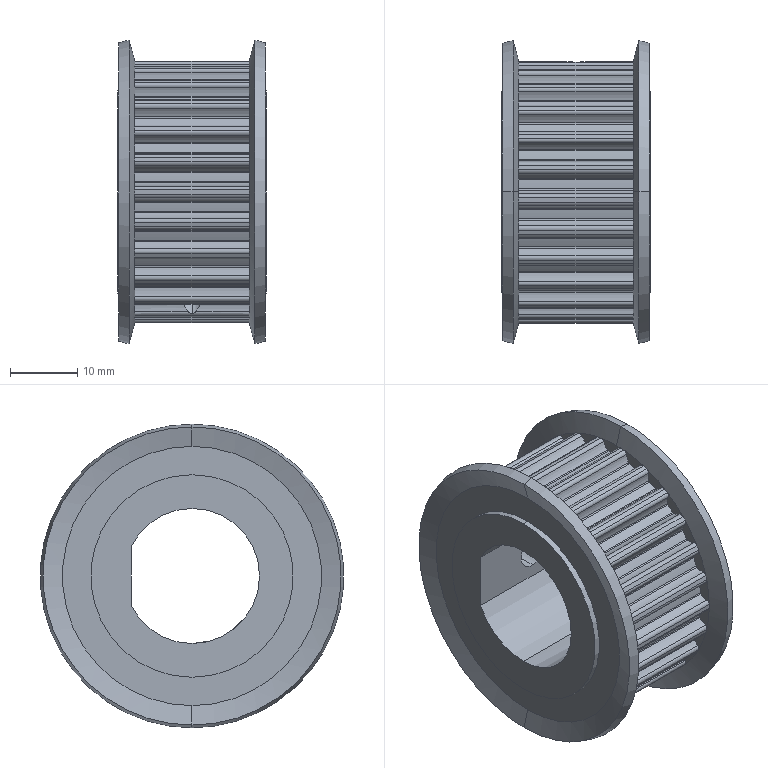Part | SolidWorks | features BaseBody 1 | 1 solid | 290 faces | box 22 x 45 x 45 mm | volume 17406 mm3 | cylinder 223 | plane 55 | cone 12 | commonest cylinder face diameters 0.5 x54 6.55 x54 1.1 x52 35.29 x27 38.83 x25 30 x4